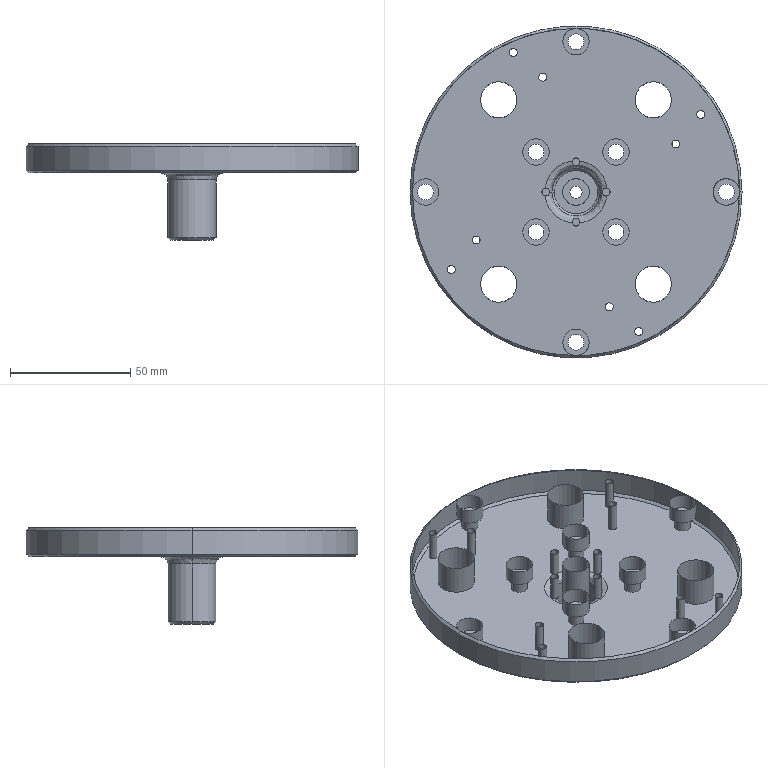Part | STEP file | Flange-market | 1 solid | 96 faces | box 138 x 138 x 40 mm | volume 168413 mm3 | cylinder 72 | plane 16 | cone 6 | spline 2 | commonest cylinder face diameters 3.3 x24 6.6 x16 11 x16 15 x8 5.1 x2 11.1 x2